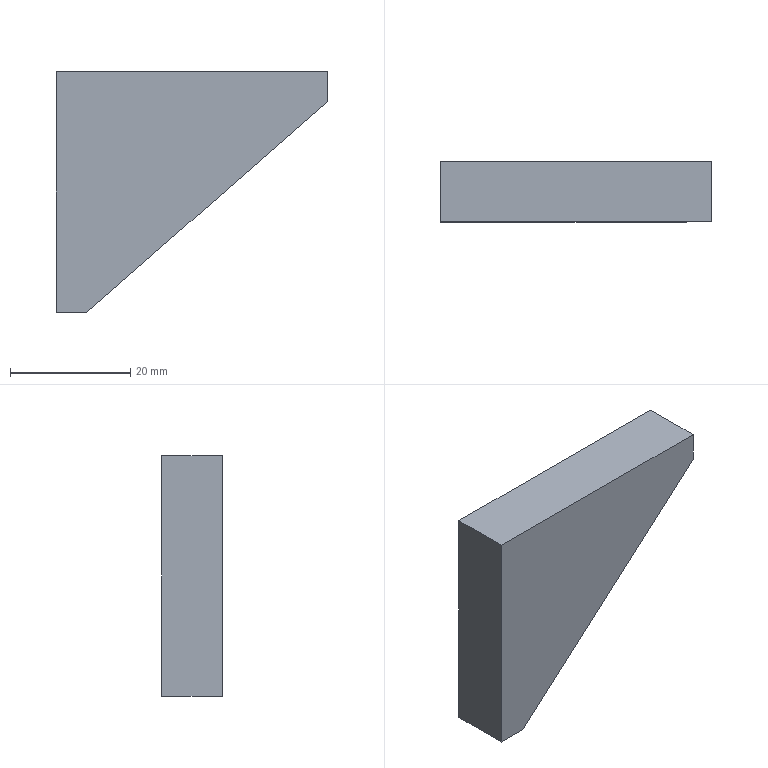Part | SolidWorks | features Extrusion 1, ICE 1 | 1 solid | 7 faces | box 45 x 10 x 40 mm | volume 11000 mm3 | plane 7
STEP:
#1=CARTESIAN_POINT('',(22.5,0.,20.));
#2=VERTEX_POINT('',#1);
#3=CARTESIAN_POINT('',(22.5,0.,15.));
#4=VERTEX_POINT('',#3);
#5=CARTESIAN_POINT('',(22.5,0.,-20.));
#6=DIRECTION('',(0.,0.,-1.));
#7=VECTOR('',#6,1000.);
#8=LINE('',#5,#7);
#9=EDGE_CURVE('',#2,#4,#8,.T.);
#10=ORIENTED_EDGE('',*,*,#9,.T.);
#11=CARTESIAN_POINT('',(22.5,10.,15.));
#12=VERTEX_POINT('',#11);
#13=CARTESIAN_POINT('',(22.5,-10.,15.));
#14=DIRECTION('',(0.,1.,0.));
#15=VECTOR('',#14,1000.);
#16=LINE('',#13,#15);
#17=EDGE_CURVE('',#4,#12,#16,.T.);
#18=ORIENTED_EDGE('',*,*,#17,.T.);
#19=CARTESIAN_POINT('',(22.5,10.,20.));
#20=VERTEX_POINT('',#19);
#21=CARTESIAN_POINT('',(22.5,10.,-20.));
#22=DIRECTION('',(0.,0.,-1.));
#23=VECTOR('',#22,1000.);
#24=LINE('',#21,#23);
#25=EDGE_CURVE('',#20,#12,#24,.T.);
#26=ORIENTED_EDGE('',*,*,#25,.F.);
#27=CARTESIAN_POINT('',(22.5,10.,20.));
#28=DIRECTION('',(0.,-1.,0.));
#29=VECTOR('',#28,1000.);
#30=LINE('',#27,#29);
#31=EDGE_CURVE('',#20,#2,#30,.T.);
#32=ORIENTED_EDGE('',*,*,#31,.T.);
#33=EDGE_LOOP('',(#10,#18,#26,#32));
#34=FACE_OUTER_BOUND('',#33,.T.);
#35=CARTESIAN_POINT('',(22.5,10.,-20.));
#36=DIRECTION('',(-1.,0.,0.));
#37=DIRECTION('',(0.,0.,1.));
#38=AXIS2_PLACEMENT_3D('',#35,#36,#37);
#39=PLANE('',#38);
#40=ADVANCED_FACE('',(#34),#39,.F.);
#41=CARTESIAN_POINT('',(-17.5,10.,-20.));
#42=VERTEX_POINT('',#41);
#43=CARTESIAN_POINT('',(-22.5,10.,-20.));
#44=VERTEX_POINT('',#43);
#45=CARTESIAN_POINT('',(-22.5,10.,-20.));
#46=DIRECTION('',(-1.,0.,0.));
#47=VECTOR('',#46,1000.);
#48=LINE('',#45,#47);
#49=EDGE_CURVE('',#42,#44,#48,.T.);
#50=ORIENTED_EDGE('',*,*,#49,.F.);
#51=CARTESIAN_POINT('',(-17.5,0.,-20.));
#52=VERTEX_POINT('',#51);
#53=CARTESIAN_POINT('',(-17.5,-10.,-20.));
#54=DIRECTION('',(0.,1.,0.));
#55=VECTOR('',#54,1000.);
#56=LINE('',#53,#55);
#57=EDGE_CURVE('',#52,#42,#56,.T.);
#58=ORIENTED_EDGE('',*,*,#57,.F.);
#59=CARTESIAN_POINT('',(-22.5,0.,-20.));
#60=VERTEX_POINT('',#59);
#61=CARTESIAN_POINT('',(-22.5,0.,-20.));
#62=DIRECTION('',(-1.,0.,0.));
#63=VECTOR('',#62,1000.);
#64=LINE('',#61,#63);
#65=EDGE_CURVE('',#52,#60,#64,.T.);
#66=ORIENTED_EDGE('',*,*,#65,.T.);
#67=CARTESIAN_POINT('',(-22.5,10.,-20.));
#68=DIRECTION('',(0.,-1.,0.));
#69=VECTOR('',#68,1000.);
#70=LINE('',#67,#69);
#71=EDGE_CURVE('',#44,#60,#70,.T.);
#72=ORIENTED_EDGE('',*,*,#71,.F.);
#73=EDGE_LOOP('',(#50,#58,#66,#72));
#74=FACE_OUTER_BOUND('',#73,.T.);
#75=CARTESIAN_POINT('',(-22.5,10.,-20.));
#76=DIRECTION('',(0.,0.,1.));
#77=DIRECTION('',(1.,0.,0.));
#78=AXIS2_PLACEMENT_3D('',#75,#76,#77);
#79=PLANE('',#78);
#80=ADVANCED_FACE('',(#74),#79,.F.);
#81=CARTESIAN_POINT('',(-22.5,0.,20.));
#82=VERTEX_POINT('',#81);
#83=CARTESIAN_POINT('',(-22.5,0.,-20.));
#84=DIRECTION('',(0.,0.,1.));
#85=VECTOR('',#84,1000.);
#86=LINE('',#83,#85);
#87=EDGE_CURVE('',#60,#82,#86,.T.);
#88=ORIENTED_EDGE('',*,*,#87,.T.);
#89=CARTESIAN_POINT('',(-22.5,10.,20.));
#90=VERTEX_POINT('',#89);
#91=CARTESIAN_POINT('',(-22.5,10.,20.));
#92=DIRECTION('',(0.,-1.,0.));
#93=VECTOR('',#92,1000.);
#94=LINE('',#91,#93);
#95=EDGE_CURVE('',#90,#82,#94,.T.);
#96=ORIENTED_EDGE('',*,*,#95,.F.);
#97=CARTESIAN_POINT('',(-22.5,10.,-20.));
#98=DIRECTION('',(0.,0.,1.));
#99=VECTOR('',#98,1000.);
#100=LINE('',#97,#99);
#101=EDGE_CURVE('',#44,#90,#100,.T.);
#102=ORIENTED_EDGE('',*,*,#101,.F.);
#103=ORIENTED_EDGE('',*,*,#71,.T.);
#104=EDGE_LOOP('',(#88,#96,#102,#103));
#105=FACE_OUTER_BOUND('',#104,.T.);
#106=CARTESIAN_POINT('',(-22.5,10.,-20.));
#107=DIRECTION('',(1.,0.,0.));
#108=DIRECTION('',(0.,0.,-1.));
#109=AXIS2_PLACEMENT_3D('',#106,#107,#108);
#110=PLANE('',#109);
#111=ADVANCED_FACE('',(#105),#110,.F.);
#112=CARTESIAN_POINT('',(-22.5,0.,20.));
#113=DIRECTION('',(1.,0.,0.));
#114=VECTOR('',#113,1000.);
#115=LINE('',#112,#114);
#116=EDGE_CURVE('',#82,#2,#115,.T.);
#117=ORIENTED_EDGE('',*,*,#116,.T.);
#118=ORIENTED_EDGE('',*,*,#31,.F.);
#119=CARTESIAN_POINT('',(-22.5,10.,20.));
#120=DIRECTION('',(1.,0.,0.));
#121=VECTOR('',#120,1000.);
#122=LINE('',#119,#121);
#123=EDGE_CURVE('',#90,#20,#122,.T.);
#124=ORIENTED_EDGE('',*,*,#123,.F.);
#125=ORIENTED_EDGE('',*,*,#95,.T.);
#126=EDGE_LOOP('',(#117,#118,#124,#125));
#127=FACE_OUTER_BOUND('',#126,.T.);
#128=CARTESIAN_POINT('',(-22.5,10.,20.));
#129=DIRECTION('',(0.,0.,-1.));
#130=DIRECTION('',(-1.,0.,0.));
#131=AXIS2_PLACEMENT_3D('',#128,#129,#130);
#132=PLANE('',#131);
#133=ADVANCED_FACE('',(#127),#132,.F.);
#134=CARTESIAN_POINT('',(-17.5,10.,-20.));
#135=DIRECTION('',(0.7526,0.,0.6585));
#136=VECTOR('',#135,1000.);
#137=LINE('',#134,#136);
#138=EDGE_CURVE('',#42,#12,#137,.T.);
#139=ORIENTED_EDGE('',*,*,#138,.F.);
#140=ORIENTED_EDGE('',*,*,#49,.T.);
#141=ORIENTED_EDGE('',*,*,#101,.T.);
#142=ORIENTED_EDGE('',*,*,#123,.T.);
#143=ORIENTED_EDGE('',*,*,#25,.T.);
#144=EDGE_LOOP('',(#139,#140,#141,#142,#143));
#145=FACE_OUTER_BOUND('',#144,.T.);
#146=CARTESIAN_POINT('',(0.,10.,0.));
#147=DIRECTION('',(0.,1.,0.));
#148=DIRECTION('',(0.,0.,1.));
#149=AXIS2_PLACEMENT_3D('',#146,#147,#148);
#150=PLANE('',#149);
#151=ADVANCED_FACE('',(#145),#150,.T.);
#152=ORIENTED_EDGE('',*,*,#65,.F.);
#153=CARTESIAN_POINT('',(2.323,0.,-2.655));
#154=DIRECTION('',(0.7526,0.,0.6585));
#155=VECTOR('',#154,1000.);
#156=LINE('',#153,#155);
#157=EDGE_CURVE('',#52,#4,#156,.T.);
#158=ORIENTED_EDGE('',*,*,#157,.T.);
#159=ORIENTED_EDGE('',*,*,#9,.F.);
#160=ORIENTED_EDGE('',*,*,#116,.F.);
#161=ORIENTED_EDGE('',*,*,#87,.F.);
#162=EDGE_LOOP('',(#152,#158,#159,#160,#161));
#163=FACE_OUTER_BOUND('',#162,.T.);
#164=CARTESIAN_POINT('',(0.,0.,0.));
#165=DIRECTION('',(0.,1.,0.));
#166=DIRECTION('',(0.,0.,1.));
#167=AXIS2_PLACEMENT_3D('',#164,#165,#166);
#168=PLANE('',#167);
#169=ADVANCED_FACE('',(#163),#168,.F.);
#170=ORIENTED_EDGE('',*,*,#57,.T.);
#171=ORIENTED_EDGE('',*,*,#138,.T.);
#172=ORIENTED_EDGE('',*,*,#17,.F.);
#173=ORIENTED_EDGE('',*,*,#157,.F.);
#174=EDGE_LOOP('',(#170,#171,#172,#173));
#175=FACE_OUTER_BOUND('',#174,.T.);
#176=CARTESIAN_POINT('',(-17.5,-10.,-20.));
#177=DIRECTION('',(-0.6585,0.,0.7526));
#178=DIRECTION('',(0.7526,0.,0.6585));
#179=AXIS2_PLACEMENT_3D('',#176,#177,#178);
#180=PLANE('',#179);
#181=ADVANCED_FACE('',(#175),#180,.F.);
#182=CLOSED_SHELL('',(#40,#80,#111,#133,#151,#169,#181));
#183=MANIFOLD_SOLID_BREP('',#182);
#184=CARTESIAN_POINT('',(0.,0.,0.));
#185=DIRECTION('',(0.,0.,1.));
#186=DIRECTION('',(1.,0.,0.));
#187=AXIS2_PLACEMENT_3D('',#184,#185,#186);
#188=(LENGTH_UNIT()NAMED_UNIT(*)SI_UNIT(.MILLI.,.METRE.));
#189=UNCERTAINTY_MEASURE_WITH_UNIT(LENGTH_MEASURE(0.00001),#188,'','');
#190=(NAMED_UNIT(*)PLANE_ANGLE_UNIT()SI_UNIT($,.RADIAN.));
#191=(NAMED_UNIT(*)SI_UNIT($,.STERADIAN.)SOLID_ANGLE_UNIT());
#192=(GEOMETRIC_REPRESENTATION_CONTEXT(3)GLOBAL_UNCERTAINTY_ASSIGNED_CONTEXT((#189))GLOBAL_UNIT_ASSIGNED_CONTEXT((#188,#190,#191))REPRESENTATION_CONTEXT('',''));
#193=ADVANCED_BREP_SHAPE_REPRESENTATION('',(#183,#187),#192);